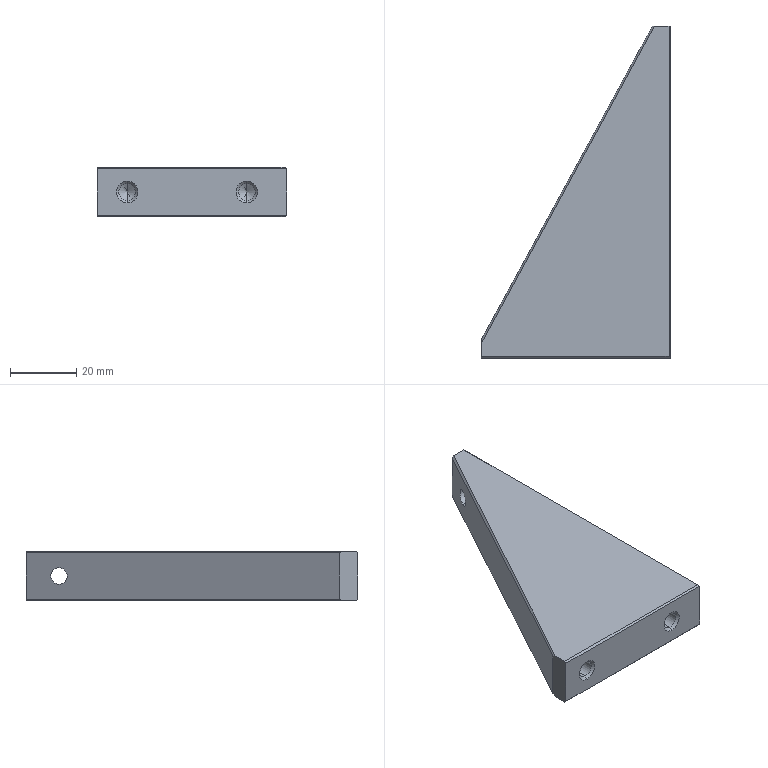Part | SolidWorks | features HoleWzd 2, Chamfer 1, Extrusion 1, ICE 1 | 1 solid | 35 faces | box 57 x 99.917 x 15 mm | volume 47753 mm3 | cone 14 | plane 13 | cylinder 8 | commonest cylinder face diameters 5 x8
STEP:
#1=CARTESIAN_POINT('',(59.493,20.,10.));
#2=VERTEX_POINT('',#1);
#3=CARTESIAN_POINT('',(59.493,20.,5.));
#4=VERTEX_POINT('',#3);
#5=CARTESIAN_POINT('',(59.493,20.,7.5));
#6=DIRECTION('',(1.,0.,0.));
#7=DIRECTION('',(0.,0.,-1.));
#8=AXIS2_PLACEMENT_3D('',#5,#6,#7);
#9=CIRCLE('',#8,2.5);
#10=EDGE_CURVE('',#2,#4,#9,.T.);
#11=ORIENTED_EDGE('',*,*,#10,.F.);
#12=CARTESIAN_POINT('',(60.,20.,10.525));
#13=VERTEX_POINT('',#12);
#14=CARTESIAN_POINT('',(60.,20.,10.525));
#15=DIRECTION('',(0.6947,0.,0.7193));
#16=VECTOR('',#15,1000.);
#17=LINE('',#14,#16);
#18=EDGE_CURVE('',#2,#13,#17,.T.);
#19=ORIENTED_EDGE('',*,*,#18,.T.);
#20=CARTESIAN_POINT('',(60.,20.,4.475));
#21=VERTEX_POINT('',#20);
#22=CARTESIAN_POINT('',(60.,20.,7.5));
#23=DIRECTION('',(1.,0.,0.));
#24=DIRECTION('',(0.,0.,-1.));
#25=AXIS2_PLACEMENT_3D('',#22,#23,#24);
#26=CIRCLE('',#25,3.025);
#27=EDGE_CURVE('',#13,#21,#26,.T.);
#28=ORIENTED_EDGE('',*,*,#27,.T.);
#29=CARTESIAN_POINT('',(60.,20.,4.475));
#30=DIRECTION('',(0.6947,0.,-0.7193));
#31=VECTOR('',#30,1000.);
#32=LINE('',#29,#31);
#33=EDGE_CURVE('',#4,#21,#32,.T.);
#34=ORIENTED_EDGE('',*,*,#33,.F.);
#35=EDGE_LOOP('',(#11,#19,#28,#34));
#36=FACE_OUTER_BOUND('',#35,.T.);
#37=CARTESIAN_POINT('',(60.,20.,7.5));
#38=DIRECTION('',(1.,0.,0.));
#39=DIRECTION('',(0.,0.,-1.));
#40=AXIS2_PLACEMENT_3D('',#37,#38,#39);
#41=CONICAL_SURFACE('',#40,3.025,0.8029);
#42=ADVANCED_FACE('',(#36),#41,.F.);
#43=CARTESIAN_POINT('',(45.,20.,10.));
#44=VERTEX_POINT('',#43);
#45=CARTESIAN_POINT('',(45.,20.,5.));
#46=VERTEX_POINT('',#45);
#47=CARTESIAN_POINT('',(45.,20.,7.5));
#48=DIRECTION('',(1.,0.,0.));
#49=DIRECTION('',(0.,0.,-1.));
#50=AXIS2_PLACEMENT_3D('',#47,#48,#49);
#51=CIRCLE('',#50,2.5);
#52=EDGE_CURVE('',#44,#46,#51,.T.);
#53=ORIENTED_EDGE('',*,*,#52,.F.);
#54=CARTESIAN_POINT('',(60.,20.,10.));
#55=DIRECTION('',(1.,0.,0.));
#56=VECTOR('',#55,1000.);
#57=LINE('',#54,#56);
#58=EDGE_CURVE('',#44,#2,#57,.T.);
#59=ORIENTED_EDGE('',*,*,#58,.T.);
#60=ORIENTED_EDGE('',*,*,#10,.T.);
#61=CARTESIAN_POINT('',(60.,20.,5.));
#62=DIRECTION('',(1.,0.,0.));
#63=VECTOR('',#62,1000.);
#64=LINE('',#61,#63);
#65=EDGE_CURVE('',#46,#4,#64,.T.);
#66=ORIENTED_EDGE('',*,*,#65,.F.);
#67=EDGE_LOOP('',(#53,#59,#60,#66));
#68=FACE_OUTER_BOUND('',#67,.T.);
#69=CARTESIAN_POINT('',(60.,20.,7.5));
#70=DIRECTION('',(1.,0.,0.));
#71=DIRECTION('',(0.,0.,-1.));
#72=AXIS2_PLACEMENT_3D('',#69,#70,#71);
#73=CYLINDRICAL_SURFACE('',#72,2.5);
#74=ADVANCED_FACE('',(#68),#73,.F.);
#75=CARTESIAN_POINT('',(43.498,20.,7.5));
#76=VERTEX_POINT('',#75);
#77=CARTESIAN_POINT('',(45.,20.,5.));
#78=DIRECTION('',(0.515,0.,-0.8572));
#79=VECTOR('',#78,1000.);
#80=LINE('',#77,#79);
#81=EDGE_CURVE('',#76,#46,#80,.T.);
#82=ORIENTED_EDGE('',*,*,#81,.F.);
#83=CARTESIAN_POINT('',(45.,20.,10.));
#84=DIRECTION('',(0.515,0.,0.8572));
#85=VECTOR('',#84,1000.);
#86=LINE('',#83,#85);
#87=EDGE_CURVE('',#76,#44,#86,.T.);
#88=ORIENTED_EDGE('',*,*,#87,.T.);
#89=ORIENTED_EDGE('',*,*,#52,.T.);
#90=EDGE_LOOP('',(#82,#88,#89));
#91=FACE_OUTER_BOUND('',#90,.T.);
#92=CARTESIAN_POINT('',(45.,20.,7.5));
#93=DIRECTION('',(1.,0.,0.));
#94=DIRECTION('',(0.,0.,-1.));
#95=AXIS2_PLACEMENT_3D('',#92,#93,#94);
#96=CONICAL_SURFACE('',#95,2.5,1.03);
#97=ADVANCED_FACE('',(#91),#96,.F.);
#98=CARTESIAN_POINT('',(59.493,90.,10.));
#99=VERTEX_POINT('',#98);
#100=CARTESIAN_POINT('',(59.493,90.,5.));
#101=VERTEX_POINT('',#100);
#102=CARTESIAN_POINT('',(59.493,90.,7.5));
#103=DIRECTION('',(1.,0.,0.));
#104=DIRECTION('',(0.,0.,-1.));
#105=AXIS2_PLACEMENT_3D('',#102,#103,#104);
#106=CIRCLE('',#105,2.5);
#107=EDGE_CURVE('',#99,#101,#106,.T.);
#108=ORIENTED_EDGE('',*,*,#107,.F.);
#109=CARTESIAN_POINT('',(60.,90.,10.525));
#110=VERTEX_POINT('',#109);
#111=CARTESIAN_POINT('',(60.,90.,10.525));
#112=DIRECTION('',(0.6947,0.,0.7193));
#113=VECTOR('',#112,1000.);
#114=LINE('',#111,#113);
#115=EDGE_CURVE('',#99,#110,#114,.T.);
#116=ORIENTED_EDGE('',*,*,#115,.T.);
#117=CARTESIAN_POINT('',(60.,90.,4.475));
#118=VERTEX_POINT('',#117);
#119=CARTESIAN_POINT('',(60.,90.,7.5));
#120=DIRECTION('',(1.,0.,0.));
#121=DIRECTION('',(0.,0.,-1.));
#122=AXIS2_PLACEMENT_3D('',#119,#120,#121);
#123=CIRCLE('',#122,3.025);
#124=EDGE_CURVE('',#110,#118,#123,.T.);
#125=ORIENTED_EDGE('',*,*,#124,.T.);
#126=CARTESIAN_POINT('',(60.,90.,4.475));
#127=DIRECTION('',(0.6947,0.,-0.7193));
#128=VECTOR('',#127,1000.);
#129=LINE('',#126,#128);
#130=EDGE_CURVE('',#101,#118,#129,.T.);
#131=ORIENTED_EDGE('',*,*,#130,.F.);
#132=EDGE_LOOP('',(#108,#116,#125,#131));
#133=FACE_OUTER_BOUND('',#132,.T.);
#134=CARTESIAN_POINT('',(60.,90.,7.5));
#135=DIRECTION('',(1.,0.,0.));
#136=DIRECTION('',(0.,0.,-1.));
#137=AXIS2_PLACEMENT_3D('',#134,#135,#136);
#138=CONICAL_SURFACE('',#137,3.025,0.8029);
#139=ADVANCED_FACE('',(#133),#138,.F.);
#140=CARTESIAN_POINT('',(49.091,90.,10.));
#141=VERTEX_POINT('',#140);
#142=CARTESIAN_POINT('',(49.091,90.,5.));
#143=VERTEX_POINT('',#142);
#144=CARTESIAN_POINT('',(49.091,90.,10.));
#145=CARTESIAN_POINT('',(46.364,85.,10.));
#146=CARTESIAN_POINT('',(46.364,85.,5.));
#147=CARTESIAN_POINT('',(49.091,90.,5.));
#148=(BOUNDED_CURVE()B_SPLINE_CURVE(3,(#144,#145,#146,#147),.UNSPECIFIED.,.F.,.F.)B_SPLINE_CURVE_WITH_KNOTS((4,4),(1.571,4.712),.UNSPECIFIED.)CURVE()GEOMETRIC_REPRESENTATION_ITEM()RATIONAL_B_SPLINE_CURVE((1.,0.3333,0.3333,1.))REPRESENTATION_ITEM(''));
#149=EDGE_CURVE('',#141,#143,#148,.T.);
#150=ORIENTED_EDGE('',*,*,#149,.F.);
#151=CARTESIAN_POINT('',(60.,90.,10.));
#152=DIRECTION('',(1.,0.,0.));
#153=VECTOR('',#152,1000.);
#154=LINE('',#151,#153);
#155=EDGE_CURVE('',#141,#99,#154,.T.);
#156=ORIENTED_EDGE('',*,*,#155,.T.);
#157=ORIENTED_EDGE('',*,*,#107,.T.);
#158=CARTESIAN_POINT('',(60.,90.,5.));
#159=DIRECTION('',(1.,0.,0.));
#160=VECTOR('',#159,1000.);
#161=LINE('',#158,#160);
#162=EDGE_CURVE('',#143,#101,#161,.T.);
#163=ORIENTED_EDGE('',*,*,#162,.F.);
#164=EDGE_LOOP('',(#150,#156,#157,#163));
#165=FACE_OUTER_BOUND('',#164,.T.);
#166=CARTESIAN_POINT('',(60.,90.,7.5));
#167=DIRECTION('',(1.,0.,0.));
#168=DIRECTION('',(0.,0.,-1.));
#169=AXIS2_PLACEMENT_3D('',#166,#167,#168);
#170=CYLINDRICAL_SURFACE('',#169,2.5);
#171=ADVANCED_FACE('',(#165),#170,.F.);
#172=CARTESIAN_POINT('',(48.,0.7243,10.));
#173=VERTEX_POINT('',#172);
#174=CARTESIAN_POINT('',(48.,0.7243,5.));
#175=VERTEX_POINT('',#174);
#176=CARTESIAN_POINT('',(48.,0.7243,7.5));
#177=DIRECTION('',(0.,-1.,0.));
#178=DIRECTION('',(0.,0.,-1.));
#179=AXIS2_PLACEMENT_3D('',#176,#177,#178);
#180=CIRCLE('',#179,2.5);
#181=EDGE_CURVE('',#173,#175,#180,.T.);
#182=ORIENTED_EDGE('',*,*,#181,.F.);
#183=CARTESIAN_POINT('',(48.,0.,10.75));
#184=VERTEX_POINT('',#183);
#185=CARTESIAN_POINT('',(48.,0.,10.75));
#186=DIRECTION('',(0.,-0.6947,0.7193));
#187=VECTOR('',#186,1000.);
#188=LINE('',#185,#187);
#189=EDGE_CURVE('',#173,#184,#188,.T.);
#190=ORIENTED_EDGE('',*,*,#189,.T.);
#191=CARTESIAN_POINT('',(48.,0.,4.25));
#192=VERTEX_POINT('',#191);
#193=CARTESIAN_POINT('',(48.,0.,7.5));
#194=DIRECTION('',(0.,-1.,0.));
#195=DIRECTION('',(0.,0.,-1.));
#196=AXIS2_PLACEMENT_3D('',#193,#194,#195);
#197=CIRCLE('',#196,3.25);
#198=EDGE_CURVE('',#184,#192,#197,.T.);
#199=ORIENTED_EDGE('',*,*,#198,.T.);
#200=CARTESIAN_POINT('',(48.,0.,4.25));
#201=DIRECTION('',(0.,-0.6947,-0.7193));
#202=VECTOR('',#201,1000.);
#203=LINE('',#200,#202);
#204=EDGE_CURVE('',#175,#192,#203,.T.);
#205=ORIENTED_EDGE('',*,*,#204,.F.);
#206=EDGE_LOOP('',(#182,#190,#199,#205));
#207=FACE_OUTER_BOUND('',#206,.T.);
#208=CARTESIAN_POINT('',(48.,0.,7.5));
#209=DIRECTION('',(0.,-1.,0.));
#210=DIRECTION('',(0.,0.,-1.));
#211=AXIS2_PLACEMENT_3D('',#208,#209,#210);
#212=CONICAL_SURFACE('',#211,3.25,0.8029);
#213=ADVANCED_FACE('',(#207),#212,.F.);
#214=CARTESIAN_POINT('',(48.,15.,10.));
#215=VERTEX_POINT('',#214);
#216=CARTESIAN_POINT('',(48.,15.,5.));
#217=VERTEX_POINT('',#216);
#218=CARTESIAN_POINT('',(48.,15.,7.5));
#219=DIRECTION('',(0.,-1.,0.));
#220=DIRECTION('',(0.,0.,-1.));
#221=AXIS2_PLACEMENT_3D('',#218,#219,#220);
#222=CIRCLE('',#221,2.5);
#223=EDGE_CURVE('',#215,#217,#222,.T.);
#224=ORIENTED_EDGE('',*,*,#223,.F.);
#225=CARTESIAN_POINT('',(48.,0.,10.));
#226=DIRECTION('',(0.,-1.,0.));
#227=VECTOR('',#226,1000.);
#228=LINE('',#225,#227);
#229=EDGE_CURVE('',#215,#173,#228,.T.);
#230=ORIENTED_EDGE('',*,*,#229,.T.);
#231=ORIENTED_EDGE('',*,*,#181,.T.);
#232=CARTESIAN_POINT('',(48.,0.,5.));
#233=DIRECTION('',(0.,-1.,0.));
#234=VECTOR('',#233,1000.);
#235=LINE('',#232,#234);
#236=EDGE_CURVE('',#217,#175,#235,.T.);
#237=ORIENTED_EDGE('',*,*,#236,.F.);
#238=EDGE_LOOP('',(#224,#230,#231,#237));
#239=FACE_OUTER_BOUND('',#238,.T.);
#240=CARTESIAN_POINT('',(48.,0.,7.5));
#241=DIRECTION('',(0.,-1.,0.));
#242=DIRECTION('',(0.,0.,-1.));
#243=AXIS2_PLACEMENT_3D('',#240,#241,#242);
#244=CYLINDRICAL_SURFACE('',#243,2.5);
#245=ADVANCED_FACE('',(#239),#244,.F.);
#246=CARTESIAN_POINT('',(48.,16.502,7.5));
#247=VERTEX_POINT('',#246);
#248=CARTESIAN_POINT('',(48.,15.,5.));
#249=DIRECTION('',(0.,-0.515,-0.8572));
#250=VECTOR('',#249,1000.);
#251=LINE('',#248,#250);
#252=EDGE_CURVE('',#247,#217,#251,.T.);
#253=ORIENTED_EDGE('',*,*,#252,.F.);
#254=CARTESIAN_POINT('',(48.,15.,10.));
#255=DIRECTION('',(0.,-0.515,0.8572));
#256=VECTOR('',#255,1000.);
#257=LINE('',#254,#256);
#258=EDGE_CURVE('',#247,#215,#257,.T.);
#259=ORIENTED_EDGE('',*,*,#258,.T.);
#260=ORIENTED_EDGE('',*,*,#223,.T.);
#261=EDGE_LOOP('',(#253,#259,#260));
#262=FACE_OUTER_BOUND('',#261,.T.);
#263=CARTESIAN_POINT('',(48.,15.,7.5));
#264=DIRECTION('',(0.,-1.,0.));
#265=DIRECTION('',(0.,0.,-1.));
#266=AXIS2_PLACEMENT_3D('',#263,#264,#265);
#267=CONICAL_SURFACE('',#266,2.5,1.03);
#268=ADVANCED_FACE('',(#262),#267,.F.);
#269=CARTESIAN_POINT('',(12.,0.7243,10.));
#270=VERTEX_POINT('',#269);
#271=CARTESIAN_POINT('',(12.,0.7243,5.));
#272=VERTEX_POINT('',#271);
#273=CARTESIAN_POINT('',(12.,0.7243,7.5));
#274=DIRECTION('',(0.,-1.,0.));
#275=DIRECTION('',(0.,0.,-1.));
#276=AXIS2_PLACEMENT_3D('',#273,#274,#275);
#277=CIRCLE('',#276,2.5);
#278=EDGE_CURVE('',#270,#272,#277,.T.);
#279=ORIENTED_EDGE('',*,*,#278,.F.);
#280=CARTESIAN_POINT('',(12.,0.,10.75));
#281=VERTEX_POINT('',#280);
#282=CARTESIAN_POINT('',(12.,0.,10.75));
#283=DIRECTION('',(0.,-0.6947,0.7193));
#284=VECTOR('',#283,1000.);
#285=LINE('',#282,#284);
#286=EDGE_CURVE('',#270,#281,#285,.T.);
#287=ORIENTED_EDGE('',*,*,#286,.T.);
#288=CARTESIAN_POINT('',(12.,0.,4.25));
#289=VERTEX_POINT('',#288);
#290=CARTESIAN_POINT('',(12.,0.,7.5));
#291=DIRECTION('',(0.,-1.,0.));
#292=DIRECTION('',(0.,0.,-1.));
#293=AXIS2_PLACEMENT_3D('',#290,#291,#292);
#294=CIRCLE('',#293,3.25);
#295=EDGE_CURVE('',#281,#289,#294,.T.);
#296=ORIENTED_EDGE('',*,*,#295,.T.);
#297=CARTESIAN_POINT('',(12.,0.,4.25));
#298=DIRECTION('',(0.,-0.6947,-0.7193));
#299=VECTOR('',#298,1000.);
#300=LINE('',#297,#299);
#301=EDGE_CURVE('',#272,#289,#300,.T.);
#302=ORIENTED_EDGE('',*,*,#301,.F.);
#303=EDGE_LOOP('',(#279,#287,#296,#302));
#304=FACE_OUTER_BOUND('',#303,.T.);
#305=CARTESIAN_POINT('',(12.,0.,7.5));
#306=DIRECTION('',(0.,-1.,0.));
#307=DIRECTION('',(0.,0.,-1.));
#308=AXIS2_PLACEMENT_3D('',#305,#306,#307);
#309=CONICAL_SURFACE('',#308,3.25,0.8029);
#310=ADVANCED_FACE('',(#304),#309,.F.);
#311=CARTESIAN_POINT('',(12.,15.,10.));
#312=VERTEX_POINT('',#311);
#313=CARTESIAN_POINT('',(12.,15.,5.));
#314=VERTEX_POINT('',#313);
#315=CARTESIAN_POINT('',(12.,15.,7.5));
#316=DIRECTION('',(0.,-1.,0.));
#317=DIRECTION('',(0.,0.,-1.));
#318=AXIS2_PLACEMENT_3D('',#315,#316,#317);
#319=CIRCLE('',#318,2.5);
#320=EDGE_CURVE('',#312,#314,#319,.T.);
#321=ORIENTED_EDGE('',*,*,#320,.F.);
#322=CARTESIAN_POINT('',(12.,0.,10.));
#323=DIRECTION('',(0.,-1.,0.));
#324=VECTOR('',#323,1000.);
#325=LINE('',#322,#324);
#326=EDGE_CURVE('',#312,#270,#325,.T.);
#327=ORIENTED_EDGE('',*,*,#326,.T.);
#328=ORIENTED_EDGE('',*,*,#278,.T.);
#329=CARTESIAN_POINT('',(12.,0.,5.));
#330=DIRECTION('',(0.,-1.,0.));
#331=VECTOR('',#330,1000.);
#332=LINE('',#329,#331);
#333=EDGE_CURVE('',#314,#272,#332,.T.);
#334=ORIENTED_EDGE('',*,*,#333,.F.);
#335=EDGE_LOOP('',(#321,#327,#328,#334));
#336=FACE_OUTER_BOUND('',#335,.T.);
#337=CARTESIAN_POINT('',(12.,0.,7.5));
#338=DIRECTION('',(0.,-1.,0.));
#339=DIRECTION('',(0.,0.,-1.));
#340=AXIS2_PLACEMENT_3D('',#337,#338,#339);
#341=CYLINDRICAL_SURFACE('',#340,2.5);
#342=ADVANCED_FACE('',(#336),#341,.F.);
#343=CARTESIAN_POINT('',(12.,16.502,7.5));
#344=VERTEX_POINT('',#343);
#345=CARTESIAN_POINT('',(12.,15.,5.));
#346=DIRECTION('',(0.,-0.515,-0.8572));
#347=VECTOR('',#346,1000.);
#348=LINE('',#345,#347);
#349=EDGE_CURVE('',#344,#314,#348,.T.);
#350=ORIENTED_EDGE('',*,*,#349,.F.);
#351=CARTESIAN_POINT('',(12.,15.,10.));
#352=DIRECTION('',(0.,-0.515,0.8572));
#353=VECTOR('',#352,1000.);
#354=LINE('',#351,#353);
#355=EDGE_CURVE('',#344,#312,#354,.T.);
#356=ORIENTED_EDGE('',*,*,#355,.T.);
#357=ORIENTED_EDGE('',*,*,#320,.T.);
#358=EDGE_LOOP('',(#350,#356,#357));
#359=FACE_OUTER_BOUND('',#358,.T.);
#360=CARTESIAN_POINT('',(12.,15.,7.5));
#361=DIRECTION('',(0.,-1.,0.));
#362=DIRECTION('',(0.,0.,-1.));
#363=AXIS2_PLACEMENT_3D('',#360,#361,#362);
#364=CONICAL_SURFACE('',#363,2.5,1.03);
#365=ADVANCED_FACE('',(#359),#364,.F.);
#366=CARTESIAN_POINT('',(49.091,90.,5.));
#367=CARTESIAN_POINT('',(51.818,95.,5.));
#368=CARTESIAN_POINT('',(51.818,95.,10.));
#369=CARTESIAN_POINT('',(49.091,90.,10.));
#370=(BOUNDED_CURVE()B_SPLINE_CURVE(3,(#366,#367,#368,#369),.UNSPECIFIED.,.F.,.T.)B_SPLINE_CURVE_WITH_KNOTS((4,4),(4.712,7.854),.UNSPECIFIED.)CURVE()GEOMETRIC_REPRESENTATION_ITEM()RATIONAL_B_SPLINE_CURVE((1.,0.3333,0.3333,1.))REPRESENTATION_ITEM(''));
#371=EDGE_CURVE('',#143,#141,#370,.T.);
#372=ORIENTED_EDGE('',*,*,#371,.T.);
#373=ORIENTED_EDGE('',*,*,#149,.T.);
#374=EDGE_LOOP('',(#372,#373));
#375=FACE_BOUND('',#374,.T.);
#376=CARTESIAN_POINT('',(54.5,99.917,0.5));
#377=VERTEX_POINT('',#376);
#378=CARTESIAN_POINT('',(3.,5.5,0.5));
#379=VERTEX_POINT('',#378);
#380=CARTESIAN_POINT('',(60.,110.,0.5));
#381=DIRECTION('',(-0.4789,-0.8779,0.));
#382=VECTOR('',#381,1000.);
#383=LINE('',#380,#382);
#384=EDGE_CURVE('',#377,#379,#383,.T.);
#385=ORIENTED_EDGE('',*,*,#384,.T.);
#386=CARTESIAN_POINT('',(3.,5.5,14.5));
#387=VERTEX_POINT('',#386);
#388=CARTESIAN_POINT('',(3.,5.5,15.));
#389=DIRECTION('',(0.,0.,1.));
#390=VECTOR('',#389,1000.);
#391=LINE('',#388,#390);
#392=EDGE_CURVE('',#379,#387,#391,.T.);
#393=ORIENTED_EDGE('',*,*,#392,.T.);
#394=CARTESIAN_POINT('',(54.5,99.917,14.5));
#395=VERTEX_POINT('',#394);
#396=CARTESIAN_POINT('',(60.,110.,14.5));
#397=DIRECTION('',(0.4789,0.8779,0.));
#398=VECTOR('',#397,1000.);
#399=LINE('',#396,#398);
#400=EDGE_CURVE('',#387,#395,#399,.T.);
#401=ORIENTED_EDGE('',*,*,#400,.T.);
#402=CARTESIAN_POINT('',(54.5,99.917,0.));
#403=DIRECTION('',(0.,0.,1.));
#404=VECTOR('',#403,1000.);
#405=LINE('',#402,#404);
#406=EDGE_CURVE('',#377,#395,#405,.T.);
#407=ORIENTED_EDGE('',*,*,#406,.F.);
#408=EDGE_LOOP('',(#385,#393,#401,#407));
#409=FACE_OUTER_BOUND('',#408,.T.);
#410=CARTESIAN_POINT('',(60.,110.,15.));
#411=DIRECTION('',(0.8779,-0.4789,0.));
#412=DIRECTION('',(0.4789,0.8779,0.));
#413=AXIS2_PLACEMENT_3D('',#410,#411,#412);
#414=PLANE('',#413);
#415=ADVANCED_FACE('',(#375,#409),#414,.F.);
#416=CARTESIAN_POINT('',(48.,0.,7.5));
#417=DIRECTION('',(0.,-1.,0.));
#418=DIRECTION('',(0.,0.,-1.));
#419=AXIS2_PLACEMENT_3D('',#416,#417,#418);
#420=CIRCLE('',#419,3.25);
#421=EDGE_CURVE('',#192,#184,#420,.T.);
#422=ORIENTED_EDGE('',*,*,#421,.F.);
#423=ORIENTED_EDGE('',*,*,#198,.F.);
#424=EDGE_LOOP('',(#422,#423));
#425=FACE_BOUND('',#424,.T.);
#426=CARTESIAN_POINT('',(12.,0.,7.5));
#427=DIRECTION('',(0.,-1.,0.));
#428=DIRECTION('',(0.,0.,-1.));
#429=AXIS2_PLACEMENT_3D('',#426,#427,#428);
#430=CIRCLE('',#429,3.25);
#431=EDGE_CURVE('',#289,#281,#430,.T.);
#432=ORIENTED_EDGE('',*,*,#431,.F.);
#433=ORIENTED_EDGE('',*,*,#295,.F.);
#434=EDGE_LOOP('',(#432,#433));
#435=FACE_BOUND('',#434,.T.);
#436=CARTESIAN_POINT('',(60.,0.,14.5));
#437=VERTEX_POINT('',#436);
#438=CARTESIAN_POINT('',(3.,0.,14.5));
#439=VERTEX_POINT('',#438);
#440=CARTESIAN_POINT('',(0.,0.,14.5));
#441=DIRECTION('',(-1.,0.,0.));
#442=VECTOR('',#441,1000.);
#443=LINE('',#440,#442);
#444=EDGE_CURVE('',#437,#439,#443,.T.);
#445=ORIENTED_EDGE('',*,*,#444,.T.);
#446=CARTESIAN_POINT('',(3.,0.,0.5));
#447=VERTEX_POINT('',#446);
#448=CARTESIAN_POINT('',(3.,0.,0.));
#449=DIRECTION('',(0.,0.,1.));
#450=VECTOR('',#449,1000.);
#451=LINE('',#448,#450);
#452=EDGE_CURVE('',#447,#439,#451,.T.);
#453=ORIENTED_EDGE('',*,*,#452,.F.);
#454=CARTESIAN_POINT('',(60.,0.,0.5));
#455=VERTEX_POINT('',#454);
#456=CARTESIAN_POINT('',(0.,0.,0.5));
#457=DIRECTION('',(1.,0.,0.));
#458=VECTOR('',#457,1000.);
#459=LINE('',#456,#458);
#460=EDGE_CURVE('',#447,#455,#459,.T.);
#461=ORIENTED_EDGE('',*,*,#460,.T.);
#462=CARTESIAN_POINT('',(60.,0.,15.));
#463=DIRECTION('',(0.,0.,-1.));
#464=VECTOR('',#463,1000.);
#465=LINE('',#462,#464);
#466=EDGE_CURVE('',#437,#455,#465,.T.);
#467=ORIENTED_EDGE('',*,*,#466,.F.);
#468=EDGE_LOOP('',(#445,#453,#461,#467));
#469=FACE_OUTER_BOUND('',#468,.T.);
#470=CARTESIAN_POINT('',(0.,0.,15.));
#471=DIRECTION('',(0.,1.,0.));
#472=DIRECTION('',(0.,0.,1.));
#473=AXIS2_PLACEMENT_3D('',#470,#471,#472);
#474=PLANE('',#473);
#475=ADVANCED_FACE('',(#425,#435,#469),#474,.F.);
#476=CARTESIAN_POINT('',(60.,20.,7.5));
#477=DIRECTION('',(1.,0.,0.));
#478=DIRECTION('',(0.,0.,-1.));
#479=AXIS2_PLACEMENT_3D('',#476,#477,#478);
#480=CIRCLE('',#479,3.025);
#481=EDGE_CURVE('',#21,#13,#480,.T.);
#482=ORIENTED_EDGE('',*,*,#481,.F.);
#483=ORIENTED_EDGE('',*,*,#27,.F.);
#484=EDGE_LOOP('',(#482,#483));
#485=FACE_BOUND('',#484,.T.);
#486=CARTESIAN_POINT('',(60.,90.,7.5));
#487=DIRECTION('',(1.,0.,0.));
#488=DIRECTION('',(0.,0.,-1.));
#489=AXIS2_PLACEMENT_3D('',#486,#487,#488);
#490=CIRCLE('',#489,3.025);
#491=EDGE_CURVE('',#118,#110,#490,.T.);
#492=ORIENTED_EDGE('',*,*,#491,.F.);
#493=ORIENTED_EDGE('',*,*,#124,.F.);
#494=EDGE_LOOP('',(#492,#493));
#495=FACE_BOUND('',#494,.T.);
#496=CARTESIAN_POINT('',(60.,99.917,0.5));
#497=VERTEX_POINT('',#496);
#498=CARTESIAN_POINT('',(60.,0.,0.5));
#499=DIRECTION('',(0.,1.,0.));
#500=VECTOR('',#499,1000.);
#501=LINE('',#498,#500);
#502=EDGE_CURVE('',#455,#497,#501,.T.);
#503=ORIENTED_EDGE('',*,*,#502,.T.);
#504=CARTESIAN_POINT('',(60.,99.917,14.5));
#505=VERTEX_POINT('',#504);
#506=CARTESIAN_POINT('',(60.,99.917,0.));
#507=DIRECTION('',(0.,0.,1.));
#508=VECTOR('',#507,1000.);
#509=LINE('',#506,#508);
#510=EDGE_CURVE('',#497,#505,#509,.T.);
#511=ORIENTED_EDGE('',*,*,#510,.T.);
#512=CARTESIAN_POINT('',(60.,0.,14.5));
#513=DIRECTION('',(0.,-1.,0.));
#514=VECTOR('',#513,1000.);
#515=LINE('',#512,#514);
#516=EDGE_CURVE('',#505,#437,#515,.T.);
#517=ORIENTED_EDGE('',*,*,#516,.T.);
#518=ORIENTED_EDGE('',*,*,#466,.T.);
#519=EDGE_LOOP('',(#503,#511,#517,#518));
#520=FACE_OUTER_BOUND('',#519,.T.);
#521=CARTESIAN_POINT('',(60.,0.,15.));
#522=DIRECTION('',(-1.,0.,0.));
#523=DIRECTION('',(0.,0.,1.));
#524=AXIS2_PLACEMENT_3D('',#521,#522,#523);
#525=PLANE('',#524);
#526=ADVANCED_FACE('',(#485,#495,#520),#525,.F.);
#527=CARTESIAN_POINT('',(3.,0.5,15.));
#528=VERTEX_POINT('',#527);
#529=CARTESIAN_POINT('',(3.,4.456,15.));
#530=VERTEX_POINT('',#529);
#531=CARTESIAN_POINT('',(3.,0.,15.));
#532=DIRECTION('',(0.,1.,0.));
#533=VECTOR('',#532,1000.);
#534=LINE('',#531,#533);
#535=EDGE_CURVE('',#528,#530,#534,.T.);
#536=ORIENTED_EDGE('',*,*,#535,.F.);
#537=CARTESIAN_POINT('',(59.5,0.5,15.));
#538=VERTEX_POINT('',#537);
#539=CARTESIAN_POINT('',(60.,0.5,15.));
#540=DIRECTION('',(1.,0.,0.));
#541=VECTOR('',#540,1000.);
#542=LINE('',#539,#541);
#543=EDGE_CURVE('',#528,#538,#542,.T.);
#544=ORIENTED_EDGE('',*,*,#543,.T.);
#545=CARTESIAN_POINT('',(59.5,99.917,15.));
#546=VERTEX_POINT('',#545);
#547=CARTESIAN_POINT('',(59.5,110.,15.));
#548=DIRECTION('',(0.,1.,0.));
#549=VECTOR('',#548,1000.);
#550=LINE('',#547,#549);
#551=EDGE_CURVE('',#538,#546,#550,.T.);
#552=ORIENTED_EDGE('',*,*,#551,.T.);
#553=CARTESIAN_POINT('',(55.07,99.917,15.));
#554=VERTEX_POINT('',#553);
#555=CARTESIAN_POINT('',(60.,99.917,15.));
#556=DIRECTION('',(1.,0.,0.));
#557=VECTOR('',#556,1000.);
#558=LINE('',#555,#557);
#559=EDGE_CURVE('',#554,#546,#558,.T.);
#560=ORIENTED_EDGE('',*,*,#559,.F.);
#561=CARTESIAN_POINT('',(0.4389,-0.2394,15.));
#562=DIRECTION('',(-0.4789,-0.8779,0.));
#563=VECTOR('',#562,1000.);
#564=LINE('',#561,#563);
#565=EDGE_CURVE('',#554,#530,#564,.T.);
#566=ORIENTED_EDGE('',*,*,#565,.T.);
#567=EDGE_LOOP('',(#536,#544,#552,#560,#566));
#568=FACE_OUTER_BOUND('',#567,.T.);
#569=CARTESIAN_POINT('',(0.,0.,15.));
#570=DIRECTION('',(0.,0.,1.));
#571=DIRECTION('',(1.,0.,0.));
#572=AXIS2_PLACEMENT_3D('',#569,#570,#571);
#573=PLANE('',#572);
#574=ADVANCED_FACE('',(#568),#573,.T.);
#575=CARTESIAN_POINT('',(59.5,0.5,0.));
#576=VERTEX_POINT('',#575);
#577=CARTESIAN_POINT('',(3.,0.5,0.));
#578=VERTEX_POINT('',#577);
#579=CARTESIAN_POINT('',(0.,0.5,0.));
#580=DIRECTION('',(-1.,0.,0.));
#581=VECTOR('',#580,1000.);
#582=LINE('',#579,#581);
#583=EDGE_CURVE('',#576,#578,#582,.T.);
#584=ORIENTED_EDGE('',*,*,#583,.T.);
#585=CARTESIAN_POINT('',(3.,4.456,0.));
#586=VERTEX_POINT('',#585);
#587=CARTESIAN_POINT('',(3.,0.,0.));
#588=DIRECTION('',(0.,1.,0.));
#589=VECTOR('',#588,1000.);
#590=LINE('',#587,#589);
#591=EDGE_CURVE('',#578,#586,#590,.T.);
#592=ORIENTED_EDGE('',*,*,#591,.T.);
#593=CARTESIAN_POINT('',(55.07,99.917,0.));
#594=VERTEX_POINT('',#593);
#595=CARTESIAN_POINT('',(0.4389,-0.2394,0.));
#596=DIRECTION('',(0.4789,0.8779,0.));
#597=VECTOR('',#596,1000.);
#598=LINE('',#595,#597);
#599=EDGE_CURVE('',#586,#594,#598,.T.);
#600=ORIENTED_EDGE('',*,*,#599,.T.);
#601=CARTESIAN_POINT('',(59.5,99.917,0.));
#602=VERTEX_POINT('',#601);
#603=CARTESIAN_POINT('',(60.,99.917,0.));
#604=DIRECTION('',(1.,0.,0.));
#605=VECTOR('',#604,1000.);
#606=LINE('',#603,#605);
#607=EDGE_CURVE('',#594,#602,#606,.T.);
#608=ORIENTED_EDGE('',*,*,#607,.T.);
#609=CARTESIAN_POINT('',(59.5,0.,0.));
#610=DIRECTION('',(0.,-1.,0.));
#611=VECTOR('',#610,1000.);
#612=LINE('',#609,#611);
#613=EDGE_CURVE('',#602,#576,#612,.T.);
#614=ORIENTED_EDGE('',*,*,#613,.T.);
#615=EDGE_LOOP('',(#584,#592,#600,#608,#614));
#616=FACE_OUTER_BOUND('',#615,.T.);
#617=CARTESIAN_POINT('',(0.,0.,0.));
#618=DIRECTION('',(0.,0.,1.));
#619=DIRECTION('',(1.,0.,0.));
#620=AXIS2_PLACEMENT_3D('',#617,#618,#619);
#621=PLANE('',#620);
#622=ADVANCED_FACE('',(#616),#621,.F.);
#623=ORIENTED_EDGE('',*,*,#355,.F.);
#624=ORIENTED_EDGE('',*,*,#349,.T.);
#625=CARTESIAN_POINT('',(12.,15.,7.5));
#626=DIRECTION('',(0.,-1.,0.));
#627=DIRECTION('',(0.,0.,-1.));
#628=AXIS2_PLACEMENT_3D('',#625,#626,#627);
#629=CIRCLE('',#628,2.5);
#630=EDGE_CURVE('',#314,#312,#629,.T.);
#631=ORIENTED_EDGE('',*,*,#630,.T.);
#632=EDGE_LOOP('',(#623,#624,#631));
#633=FACE_OUTER_BOUND('',#632,.T.);
#634=CARTESIAN_POINT('',(12.,15.,7.5));
#635=DIRECTION('',(0.,-1.,0.));
#636=DIRECTION('',(0.,0.,-1.));
#637=AXIS2_PLACEMENT_3D('',#634,#635,#636);
#638=CONICAL_SURFACE('',#637,2.5,1.03);
#639=ADVANCED_FACE('',(#633),#638,.F.);
#640=ORIENTED_EDGE('',*,*,#326,.F.);
#641=ORIENTED_EDGE('',*,*,#630,.F.);
#642=ORIENTED_EDGE('',*,*,#333,.T.);
#643=CARTESIAN_POINT('',(12.,0.7243,7.5));
#644=DIRECTION('',(0.,-1.,0.));
#645=DIRECTION('',(0.,0.,-1.));
#646=AXIS2_PLACEMENT_3D('',#643,#644,#645);
#647=CIRCLE('',#646,2.5);
#648=EDGE_CURVE('',#272,#270,#647,.T.);
#649=ORIENTED_EDGE('',*,*,#648,.T.);
#650=EDGE_LOOP('',(#640,#641,#642,#649));
#651=FACE_OUTER_BOUND('',#650,.T.);
#652=CARTESIAN_POINT('',(12.,0.,7.5));
#653=DIRECTION('',(0.,-1.,0.));
#654=DIRECTION('',(0.,0.,-1.));
#655=AXIS2_PLACEMENT_3D('',#652,#653,#654);
#656=CYLINDRICAL_SURFACE('',#655,2.5);
#657=ADVANCED_FACE('',(#651),#656,.F.);
#658=ORIENTED_EDGE('',*,*,#286,.F.);
#659=ORIENTED_EDGE('',*,*,#648,.F.);
#660=ORIENTED_EDGE('',*,*,#301,.T.);
#661=ORIENTED_EDGE('',*,*,#431,.T.);
#662=EDGE_LOOP('',(#658,#659,#660,#661));
#663=FACE_OUTER_BOUND('',#662,.T.);
#664=CARTESIAN_POINT('',(12.,0.,7.5));
#665=DIRECTION('',(0.,-1.,0.));
#666=DIRECTION('',(0.,0.,-1.));
#667=AXIS2_PLACEMENT_3D('',#664,#665,#666);
#668=CONICAL_SURFACE('',#667,3.25,0.8029);
#669=ADVANCED_FACE('',(#663),#668,.F.);
#670=ORIENTED_EDGE('',*,*,#258,.F.);
#671=ORIENTED_EDGE('',*,*,#252,.T.);
#672=CARTESIAN_POINT('',(48.,15.,7.5));
#673=DIRECTION('',(0.,-1.,0.));
#674=DIRECTION('',(0.,0.,-1.));
#675=AXIS2_PLACEMENT_3D('',#672,#673,#674);
#676=CIRCLE('',#675,2.5);
#677=EDGE_CURVE('',#217,#215,#676,.T.);
#678=ORIENTED_EDGE('',*,*,#677,.T.);
#679=EDGE_LOOP('',(#670,#671,#678));
#680=FACE_OUTER_BOUND('',#679,.T.);
#681=CARTESIAN_POINT('',(48.,15.,7.5));
#682=DIRECTION('',(0.,-1.,0.));
#683=DIRECTION('',(0.,0.,-1.));
#684=AXIS2_PLACEMENT_3D('',#681,#682,#683);
#685=CONICAL_SURFACE('',#684,2.5,1.03);
#686=ADVANCED_FACE('',(#680),#685,.F.);
#687=ORIENTED_EDGE('',*,*,#229,.F.);
#688=ORIENTED_EDGE('',*,*,#677,.F.);
#689=ORIENTED_EDGE('',*,*,#236,.T.);
#690=CARTESIAN_POINT('',(48.,0.7243,7.5));
#691=DIRECTION('',(0.,-1.,0.));
#692=DIRECTION('',(0.,0.,-1.));
#693=AXIS2_PLACEMENT_3D('',#690,#691,#692);
#694=CIRCLE('',#693,2.5);
#695=EDGE_CURVE('',#175,#173,#694,.T.);
#696=ORIENTED_EDGE('',*,*,#695,.T.);
#697=EDGE_LOOP('',(#687,#688,#689,#696));
#698=FACE_OUTER_BOUND('',#697,.T.);
#699=CARTESIAN_POINT('',(48.,0.,7.5));
#700=DIRECTION('',(0.,-1.,0.));
#701=DIRECTION('',(0.,0.,-1.));
#702=AXIS2_PLACEMENT_3D('',#699,#700,#701);
#703=CYLINDRICAL_SURFACE('',#702,2.5);
#704=ADVANCED_FACE('',(#698),#703,.F.);
#705=ORIENTED_EDGE('',*,*,#189,.F.);
#706=ORIENTED_EDGE('',*,*,#695,.F.);
#707=ORIENTED_EDGE('',*,*,#204,.T.);
#708=ORIENTED_EDGE('',*,*,#421,.T.);
#709=EDGE_LOOP('',(#705,#706,#707,#708));
#710=FACE_OUTER_BOUND('',#709,.T.);
#711=CARTESIAN_POINT('',(48.,0.,7.5));
#712=DIRECTION('',(0.,-1.,0.));
#713=DIRECTION('',(0.,0.,-1.));
#714=AXIS2_PLACEMENT_3D('',#711,#712,#713);
#715=CONICAL_SURFACE('',#714,3.25,0.8029);
#716=ADVANCED_FACE('',(#710),#715,.F.);
#717=ORIENTED_EDGE('',*,*,#155,.F.);
#718=ORIENTED_EDGE('',*,*,#371,.F.);
#719=ORIENTED_EDGE('',*,*,#162,.T.);
#720=CARTESIAN_POINT('',(59.493,90.,7.5));
#721=DIRECTION('',(1.,0.,0.));
#722=DIRECTION('',(0.,0.,-1.));
#723=AXIS2_PLACEMENT_3D('',#720,#721,#722);
#724=CIRCLE('',#723,2.5);
#725=EDGE_CURVE('',#101,#99,#724,.T.);
#726=ORIENTED_EDGE('',*,*,#725,.T.);
#727=EDGE_LOOP('',(#717,#718,#719,#726));
#728=FACE_OUTER_BOUND('',#727,.T.);
#729=CARTESIAN_POINT('',(60.,90.,7.5));
#730=DIRECTION('',(1.,0.,0.));
#731=DIRECTION('',(0.,0.,-1.));
#732=AXIS2_PLACEMENT_3D('',#729,#730,#731);
#733=CYLINDRICAL_SURFACE('',#732,2.5);
#734=ADVANCED_FACE('',(#728),#733,.F.);
#735=ORIENTED_EDGE('',*,*,#115,.F.);
#736=ORIENTED_EDGE('',*,*,#725,.F.);
#737=ORIENTED_EDGE('',*,*,#130,.T.);
#738=ORIENTED_EDGE('',*,*,#491,.T.);
#739=EDGE_LOOP('',(#735,#736,#737,#738));
#740=FACE_OUTER_BOUND('',#739,.T.);
#741=CARTESIAN_POINT('',(60.,90.,7.5));
#742=DIRECTION('',(1.,0.,0.));
#743=DIRECTION('',(0.,0.,-1.));
#744=AXIS2_PLACEMENT_3D('',#741,#742,#743);
#745=CONICAL_SURFACE('',#744,3.025,0.8029);
#746=ADVANCED_FACE('',(#740),#745,.F.);
#747=ORIENTED_EDGE('',*,*,#87,.F.);
#748=ORIENTED_EDGE('',*,*,#81,.T.);
#749=CARTESIAN_POINT('',(45.,20.,7.5));
#750=DIRECTION('',(1.,0.,0.));
#751=DIRECTION('',(0.,0.,-1.));
#752=AXIS2_PLACEMENT_3D('',#749,#750,#751);
#753=CIRCLE('',#752,2.5);
#754=EDGE_CURVE('',#46,#44,#753,.T.);
#755=ORIENTED_EDGE('',*,*,#754,.T.);
#756=EDGE_LOOP('',(#747,#748,#755));
#757=FACE_OUTER_BOUND('',#756,.T.);
#758=CARTESIAN_POINT('',(45.,20.,7.5));
#759=DIRECTION('',(1.,0.,0.));
#760=DIRECTION('',(0.,0.,-1.));
#761=AXIS2_PLACEMENT_3D('',#758,#759,#760);
#762=CONICAL_SURFACE('',#761,2.5,1.03);
#763=ADVANCED_FACE('',(#757),#762,.F.);
#764=ORIENTED_EDGE('',*,*,#58,.F.);
#765=ORIENTED_EDGE('',*,*,#754,.F.);
#766=ORIENTED_EDGE('',*,*,#65,.T.);
#767=CARTESIAN_POINT('',(59.493,20.,7.5));
#768=DIRECTION('',(1.,0.,0.));
#769=DIRECTION('',(0.,0.,-1.));
#770=AXIS2_PLACEMENT_3D('',#767,#768,#769);
#771=CIRCLE('',#770,2.5);
#772=EDGE_CURVE('',#4,#2,#771,.T.);
#773=ORIENTED_EDGE('',*,*,#772,.T.);
#774=EDGE_LOOP('',(#764,#765,#766,#773));
#775=FACE_OUTER_BOUND('',#774,.T.);
#776=CARTESIAN_POINT('',(60.,20.,7.5));
#777=DIRECTION('',(1.,0.,0.));
#778=DIRECTION('',(0.,0.,-1.));
#779=AXIS2_PLACEMENT_3D('',#776,#777,#778);
#780=CYLINDRICAL_SURFACE('',#779,2.5);
#781=ADVANCED_FACE('',(#775),#780,.F.);
#782=ORIENTED_EDGE('',*,*,#18,.F.);
#783=ORIENTED_EDGE('',*,*,#772,.F.);
#784=ORIENTED_EDGE('',*,*,#33,.T.);
#785=ORIENTED_EDGE('',*,*,#481,.T.);
#786=EDGE_LOOP('',(#782,#783,#784,#785));
#787=FACE_OUTER_BOUND('',#786,.T.);
#788=CARTESIAN_POINT('',(60.,20.,7.5));
#789=DIRECTION('',(1.,0.,0.));
#790=DIRECTION('',(0.,0.,-1.));
#791=AXIS2_PLACEMENT_3D('',#788,#789,#790);
#792=CONICAL_SURFACE('',#791,3.025,0.8029);
#793=ADVANCED_FACE('',(#787),#792,.F.);
#794=CARTESIAN_POINT('',(3.,90.508,41.206));
#795=DIRECTION('',(0.,-0.9019,-0.4319));
#796=VECTOR('',#795,1000.);
#797=LINE('',#794,#796);
#798=EDGE_CURVE('',#379,#586,#797,.T.);
#799=ORIENTED_EDGE('',*,*,#798,.F.);
#800=ORIENTED_EDGE('',*,*,#384,.F.);
#801=CARTESIAN_POINT('',(57.606,99.917,-2.227));
#802=DIRECTION('',(-0.7515,0.,0.6597));
#803=VECTOR('',#802,1000.);
#804=LINE('',#801,#803);
#805=EDGE_CURVE('',#594,#377,#804,.T.);
#806=ORIENTED_EDGE('',*,*,#805,.F.);
#807=ORIENTED_EDGE('',*,*,#599,.F.);
#808=EDGE_LOOP('',(#799,#800,#806,#807));
#809=FACE_OUTER_BOUND('',#808,.T.);
#810=CARTESIAN_POINT('',(60.,110.,0.5));
#811=DIRECTION('',(0.6208,-0.3386,0.7071));
#812=DIRECTION('',(-0.4789,-0.8779,0.));
#813=AXIS2_PLACEMENT_3D('',#810,#811,#812);
#814=PLANE('',#813);
#815=ADVANCED_FACE('',(#809),#814,.F.);
#816=CARTESIAN_POINT('',(60.,99.917,0.5));
#817=DIRECTION('',(-0.7071,0.,-0.7071));
#818=VECTOR('',#817,1000.);
#819=LINE('',#816,#818);
#820=EDGE_CURVE('',#497,#602,#819,.T.);
#821=ORIENTED_EDGE('',*,*,#820,.F.);
#822=ORIENTED_EDGE('',*,*,#502,.F.);
#823=CARTESIAN_POINT('',(60.,0.,0.5));
#824=DIRECTION('',(0.5774,-0.5774,0.5774));
#825=VECTOR('',#824,1000.);
#826=LINE('',#823,#825);
#827=EDGE_CURVE('',#576,#455,#826,.T.);
#828=ORIENTED_EDGE('',*,*,#827,.F.);
#829=ORIENTED_EDGE('',*,*,#613,.F.);
#830=EDGE_LOOP('',(#821,#822,#828,#829));
#831=FACE_OUTER_BOUND('',#830,.T.);
#832=CARTESIAN_POINT('',(60.,0.,0.5));
#833=DIRECTION('',(-0.7071,0.,0.7071));
#834=DIRECTION('',(0.,1.,0.));
#835=AXIS2_PLACEMENT_3D('',#832,#833,#834);
#836=PLANE('',#835);
#837=ADVANCED_FACE('',(#831),#836,.F.);
#838=CARTESIAN_POINT('',(3.,0.,0.5));
#839=DIRECTION('',(0.,-0.7071,0.7071));
#840=VECTOR('',#839,1000.);
#841=LINE('',#838,#840);
#842=EDGE_CURVE('',#578,#447,#841,.T.);
#843=ORIENTED_EDGE('',*,*,#842,.F.);
#844=ORIENTED_EDGE('',*,*,#583,.F.);
#845=ORIENTED_EDGE('',*,*,#827,.T.);
#846=ORIENTED_EDGE('',*,*,#460,.F.);
#847=EDGE_LOOP('',(#843,#844,#845,#846));
#848=FACE_OUTER_BOUND('',#847,.T.);
#849=CARTESIAN_POINT('',(0.,0.,0.5));
#850=DIRECTION('',(0.,0.7071,0.7071));
#851=DIRECTION('',(1.,0.,0.));
#852=AXIS2_PLACEMENT_3D('',#849,#850,#851);
#853=PLANE('',#852);
#854=ADVANCED_FACE('',(#848),#853,.F.);
#855=CARTESIAN_POINT('',(3.,0.5,15.));
#856=DIRECTION('',(0.,0.7071,0.7071));
#857=VECTOR('',#856,1000.);
#858=LINE('',#855,#857);
#859=EDGE_CURVE('',#439,#528,#858,.T.);
#860=ORIENTED_EDGE('',*,*,#859,.F.);
#861=ORIENTED_EDGE('',*,*,#444,.F.);
#862=CARTESIAN_POINT('',(39.667,20.333,34.833));
#863=DIRECTION('',(0.5774,-0.5774,-0.5774));
#864=VECTOR('',#863,1000.);
#865=LINE('',#862,#864);
#866=EDGE_CURVE('',#538,#437,#865,.T.);
#867=ORIENTED_EDGE('',*,*,#866,.F.);
#868=ORIENTED_EDGE('',*,*,#543,.F.);
#869=EDGE_LOOP('',(#860,#861,#867,#868));
#870=FACE_OUTER_BOUND('',#869,.T.);
#871=CARTESIAN_POINT('',(0.,0.5,15.));
#872=DIRECTION('',(0.,-0.7071,0.7071));
#873=DIRECTION('',(-1.,0.,0.));
#874=AXIS2_PLACEMENT_3D('',#871,#872,#873);
#875=PLANE('',#874);
#876=ADVANCED_FACE('',(#870),#875,.T.);
#877=CARTESIAN_POINT('',(3.,0.6364,16.829));
#878=DIRECTION('',(0.,0.9019,-0.4319));
#879=VECTOR('',#878,1000.);
#880=LINE('',#877,#879);
#881=EDGE_CURVE('',#530,#387,#880,.T.);
#882=ORIENTED_EDGE('',*,*,#881,.F.);
#883=ORIENTED_EDGE('',*,*,#565,.F.);
#884=CARTESIAN_POINT('',(24.217,99.917,-12.085));
#885=DIRECTION('',(0.7515,0.,0.6597));
#886=VECTOR('',#885,1000.);
#887=LINE('',#884,#886);
#888=EDGE_CURVE('',#395,#554,#887,.T.);
#889=ORIENTED_EDGE('',*,*,#888,.F.);
#890=ORIENTED_EDGE('',*,*,#400,.F.);
#891=EDGE_LOOP('',(#882,#883,#889,#890));
#892=FACE_OUTER_BOUND('',#891,.T.);
#893=CARTESIAN_POINT('',(0.4389,-0.2394,15.));
#894=DIRECTION('',(-0.6208,0.3386,0.7071));
#895=DIRECTION('',(0.4789,0.8779,0.));
#896=AXIS2_PLACEMENT_3D('',#893,#894,#895);
#897=PLANE('',#896);
#898=ADVANCED_FACE('',(#892),#897,.T.);
#899=CARTESIAN_POINT('',(59.5,99.917,15.));
#900=DIRECTION('',(0.7071,0.,-0.7071));
#901=VECTOR('',#900,1000.);
#902=LINE('',#899,#901);
#903=EDGE_CURVE('',#546,#505,#902,.T.);
#904=ORIENTED_EDGE('',*,*,#903,.F.);
#905=ORIENTED_EDGE('',*,*,#551,.F.);
#906=ORIENTED_EDGE('',*,*,#866,.T.);
#907=ORIENTED_EDGE('',*,*,#516,.F.);
#908=EDGE_LOOP('',(#904,#905,#906,#907));
#909=FACE_OUTER_BOUND('',#908,.T.);
#910=CARTESIAN_POINT('',(59.5,0.,15.));
#911=DIRECTION('',(0.7071,0.,0.7071));
#912=DIRECTION('',(0.,-1.,0.));
#913=AXIS2_PLACEMENT_3D('',#910,#911,#912);
#914=PLANE('',#913);
#915=ADVANCED_FACE('',(#909),#914,.T.);
#916=ORIENTED_EDGE('',*,*,#805,.T.);
#917=ORIENTED_EDGE('',*,*,#406,.T.);
#918=ORIENTED_EDGE('',*,*,#888,.T.);
#919=ORIENTED_EDGE('',*,*,#559,.T.);
#920=ORIENTED_EDGE('',*,*,#903,.T.);
#921=ORIENTED_EDGE('',*,*,#510,.F.);
#922=ORIENTED_EDGE('',*,*,#820,.T.);
#923=ORIENTED_EDGE('',*,*,#607,.F.);
#924=EDGE_LOOP('',(#916,#917,#918,#919,#920,#921,#922,#923));
#925=FACE_OUTER_BOUND('',#924,.T.);
#926=CARTESIAN_POINT('',(60.,99.917,0.));
#927=DIRECTION('',(0.,-1.,0.));
#928=DIRECTION('',(0.,0.,-1.));
#929=AXIS2_PLACEMENT_3D('',#926,#927,#928);
#930=PLANE('',#929);
#931=ADVANCED_FACE('',(#925),#930,.F.);
#932=ORIENTED_EDGE('',*,*,#842,.T.);
#933=ORIENTED_EDGE('',*,*,#452,.T.);
#934=ORIENTED_EDGE('',*,*,#859,.T.);
#935=ORIENTED_EDGE('',*,*,#535,.T.);
#936=ORIENTED_EDGE('',*,*,#881,.T.);
#937=ORIENTED_EDGE('',*,*,#392,.F.);
#938=ORIENTED_EDGE('',*,*,#798,.T.);
#939=ORIENTED_EDGE('',*,*,#591,.F.);
#940=EDGE_LOOP('',(#932,#933,#934,#935,#936,#937,#938,#939));
#941=FACE_OUTER_BOUND('',#940,.T.);
#942=CARTESIAN_POINT('',(3.,0.,0.));
#943=DIRECTION('',(1.,0.,0.));
#944=DIRECTION('',(0.,0.,-1.));
#945=AXIS2_PLACEMENT_3D('',#942,#943,#944);
#946=PLANE('',#945);
#947=ADVANCED_FACE('',(#941),#946,.F.);
#948=CLOSED_SHELL('',(#42,#74,#97,#139,#171,#213,#245,#268,#310,#342,#365,#415,#475,#526,#574,#622,#639,#657,#669,#686,#704,#716,#734,#746,#763,#781,#793,#815,#837,#854,#876,#898,#915,#931,#947));
#949=MANIFOLD_SOLID_BREP('',#948);
#950=CARTESIAN_POINT('',(0.,0.,0.));
#951=DIRECTION('',(0.,0.,1.));
#952=DIRECTION('',(1.,0.,0.));
#953=AXIS2_PLACEMENT_3D('',#950,#951,#952);
#954=(LENGTH_UNIT()NAMED_UNIT(*)SI_UNIT(.MILLI.,.METRE.));
#955=UNCERTAINTY_MEASURE_WITH_UNIT(LENGTH_MEASURE(0.00001),#954,'','');
#956=(NAMED_UNIT(*)PLANE_ANGLE_UNIT()SI_UNIT($,.RADIAN.));
#957=(NAMED_UNIT(*)SI_UNIT($,.STERADIAN.)SOLID_ANGLE_UNIT());
#958=(GEOMETRIC_REPRESENTATION_CONTEXT(3)GLOBAL_UNCERTAINTY_ASSIGNED_CONTEXT((#955))GLOBAL_UNIT_ASSIGNED_CONTEXT((#954,#956,#957))REPRESENTATION_CONTEXT('',''));
#959=ADVANCED_BREP_SHAPE_REPRESENTATION('',(#949,#953),#958);